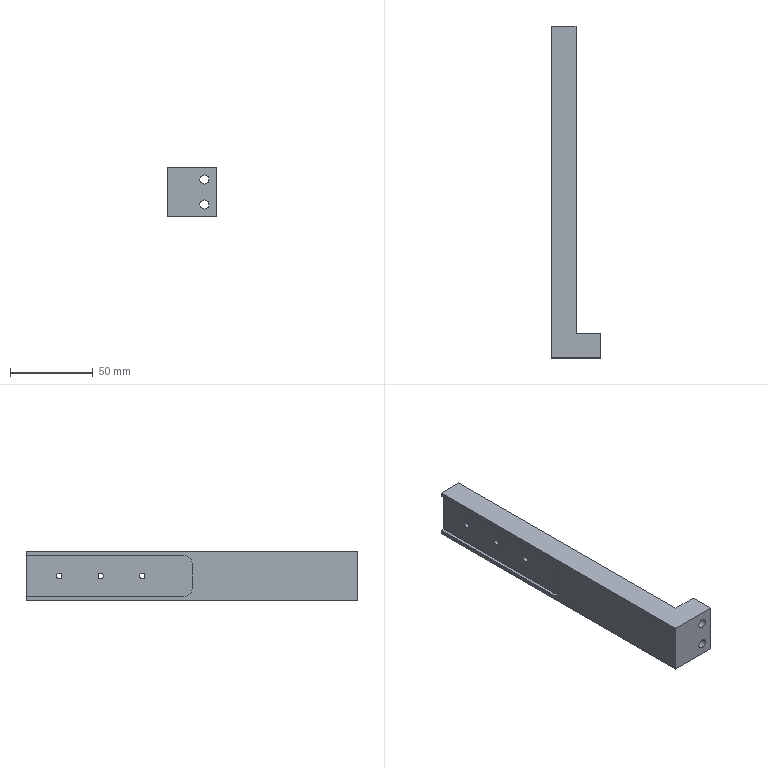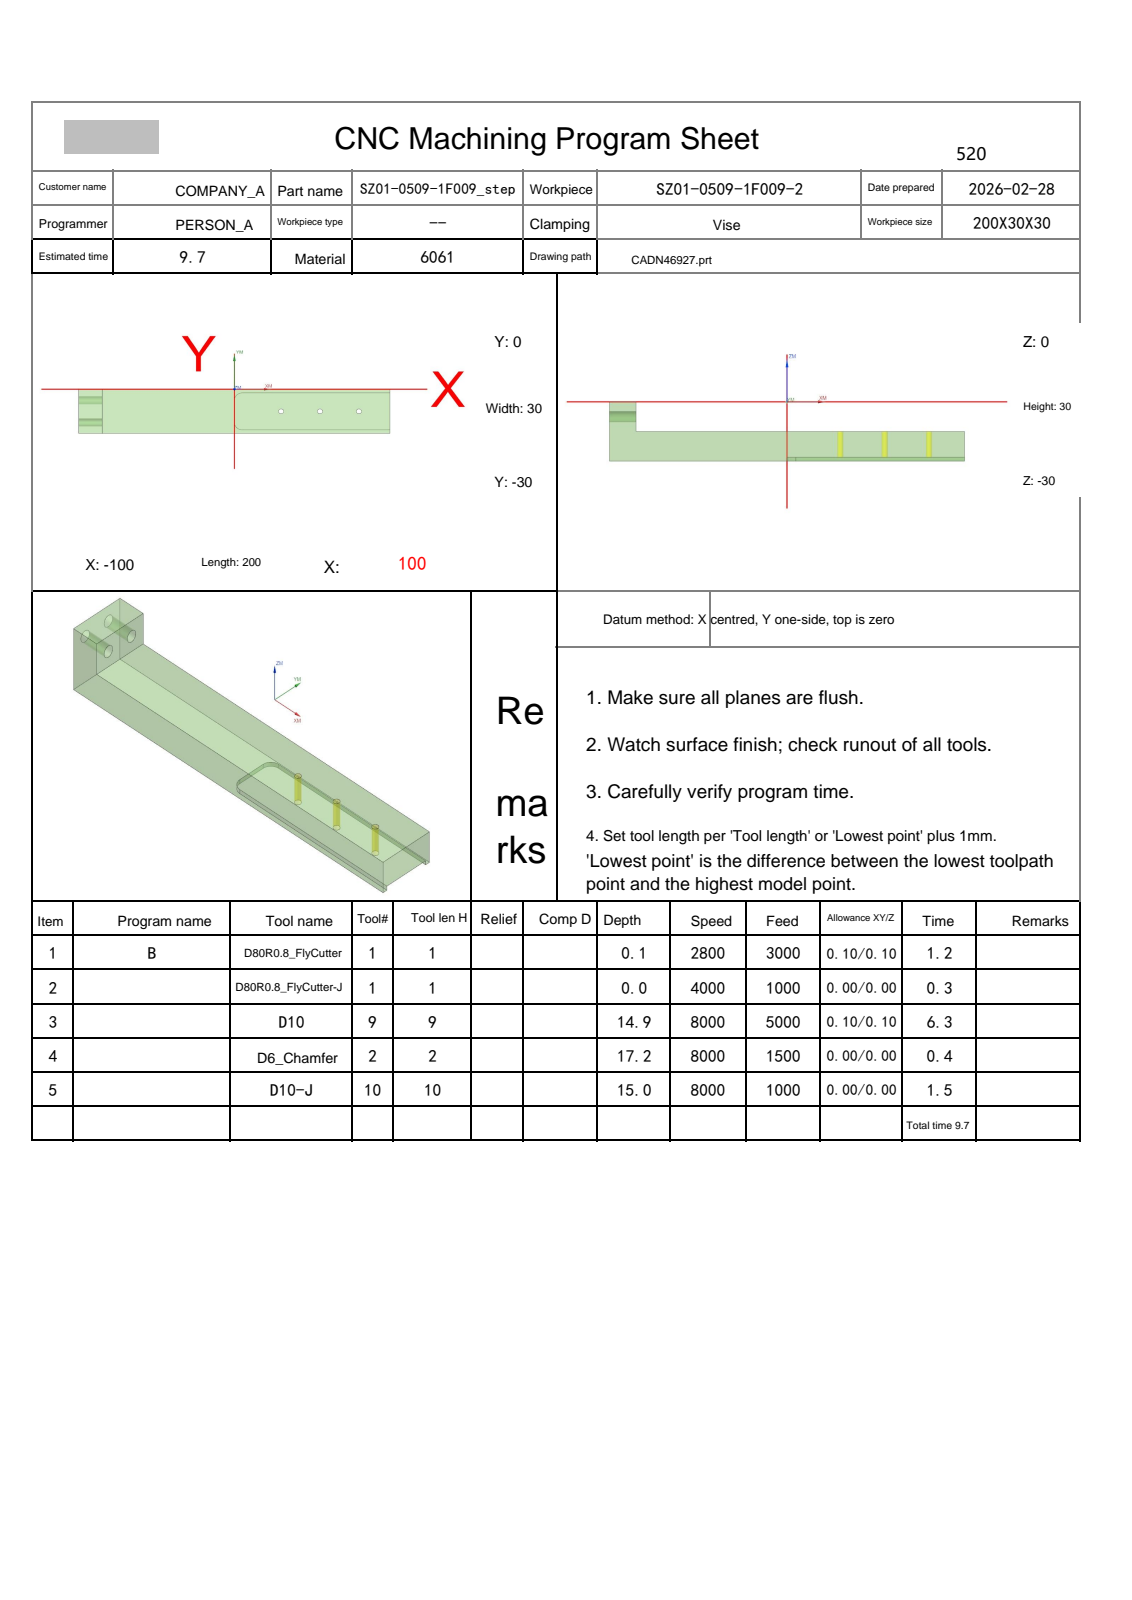NC program | NX | posted by the shop | part box 30 x 200 x 30 mm
Lines 2719 to 2890 of 2890:
N4 T02 M06
(D6_Chamfer  D=6. R=0. H=02 ce=0.00 di=0.10)
G00 G90 G54 X80. Y-15. M03 S8000
G43 H02 Z50.
M08
G98 G81 X80. Y-15. Z-17.2 R-12. F1000.
X55.
X30.
G80
G00 Z50.
G00 G90 X-83.773 Y-14.614 M03 S6500
Z50.
Z.172
G01 Z-1.2 F1500.
G03 X-83.973 Y-14.9 I1.532 J-1.286
G01 X-84.003 Y-14.946
X-84. Y-15.
Y-30.
G02 X-85. Y-31. I-1. J0.0
G01 X-100.
G02 X-101. Y-30. I0.0 J1.
G01 Y0.0
G02 X-100. Y1. I1. J0.0
G01 X-85.
G02 X-84. Y0.0 I0.0 J-1.
G01 Y-15.
X-84.003 Y-15.054
X-83.973 Y-15.1
G03 X-83.773 Y-15.386 I1.732 J1.
G01 Z.172
G00 Z10.
X-81.961 Y1.045
Z-1.815
G01 Z-16.2
X-81.904 Y1.005
X-81.884 Y1.
X100.
G02 X101. Y0.0 I0.0 J-1.
G01 Y-30.
G02 X100. Y-31. I-1. J0.0
G01 X-81.884
X-81.904 Y-31.005
X-81.961 Y-31.045
Z-1.815
G00 Z10.
X29.581 Y-15.494
Z-14.595
G01 Z-16.2
G03 X29.897 Y-15.641 I1. J1.732
G01 X29.947 Y-15.662
X30. Y-15.65
G03 X30.65 Y-15. I0.0 J.65
X30. Y-14.35 I-.65 J0.0
X29.35 Y-15. I0.0 J-.65
X30. Y-15.65 I.65 J0.0
G01 X30.053 Y-15.662
X30.103 Y-15.641
G03 X30.419 Y-15.494 I-.684 J1.879
G01 Z-14.595
G00 Z10.
X54.581
Z-14.595
G01 Z-16.2
G03 X54.897 Y-15.641 I1. J1.732
G01 X54.947 Y-15.662
X55. Y-15.65
G03 X55.65 Y-15. I0.0 J.65
X55. Y-14.35 I-.65 J0.0
X54.35 Y-15. I0.0 J-.65
X55. Y-15.65 I.65 J0.0
G01 X55.053 Y-15.662
X55.103 Y-15.641
G03 X55.419 Y-15.494 I-.684 J1.879
G01 Z-14.595
G00 Z10.
X79.581
Z-14.595
G01 Z-16.2
G03 X79.897 Y-15.641 I1. J1.732
G01 X79.947 Y-15.662
X80. Y-15.65
G03 X80.65 Y-15. I0.0 J.65
X80. Y-14.35 I-.65 J0.0
X79.35 Y-15. I0.0 J-.65
X80. Y-15.65 I.65 J0.0
G01 X80.053 Y-15.662
X80.103 Y-15.641
G03 X80.419 Y-15.494 I-.684 J1.879
G01 Z-14.595
G00 Z50.
G91 G28 Z0.0
M05
M09
G91 G28 Z0.0
M01
N5 T10 M06
(D10-J  D=10. R=0. H=10 ce=0.40 di=0.00)
G00 G90 G54 X8.7 Y7. M03 S8000
G43 H10 Z14.5
M08
Z-13.5
G01 Z-15. F1000.
Y3.
G03 X10.7 Y1. I2. J0.0
G01 X96.
X100.004
G02 X101. Y.004 I-.004 J-1.
G01 Y-30.004
G02 X100.004 Y-31. I-1. J.004
G01 X-78.604
G02 X-79.6 Y-30.004 I.004 J1.
G01 Y.004
G02 X-78.604 Y1. I1. J-.004
G01 X12.787
G02 X13.492 Y.708 I-.001 J-1.
G01 X17.908 Y-3.708
G03 X18.614 Y-4. I.707 J.708
G01 X95.004
G02 X96. Y-4.996 I-.004 J-1.
G01 Y-25.004
G02 X95.004 Y-26. I-1. J.004
G01 X-73.604
G02 X-74.6 Y-25.004 I.004 J1.
G01 Y-4.996
G02 X-73.604 Y-4. I1. J-.004
G01 X12.787
G02 X13.492 Y-4.292 I-.001 J-1.
G01 X17.908 Y-8.708
G03 X18.614 Y-9. I.707 J.708
G01 X90.004
G02 X91. Y-9.996 I-.004 J-1.
G01 Y-20.004
G02 X90.004 Y-21. I-1. J.004
G01 X-68.604
G02 X-69.6 Y-20.004 I.004 J1.
G01 Y-9.996
G02 X-68.604 Y-9. I1. J-.004
G01 X12.786
G02 X13.492 Y-9.292 I-.001 J-1.
G01 X17.908 Y-13.708
G03 X18.614 Y-14. I.707 J.708
G01 X85.005
G02 X86. Y-15. I-.005 J-1.
G01 Y-15.005
G02 X85.005 Y-16. I-1. J.005
G01 X-63.605
G02 X-64.6 Y-15. I.005 J1.
G01 Y-14.995
G02 X-63.605 Y-14. I1. J-.005
G01 X15.7
X16.7
G03 X18.7 Y-12. I0.0 J2.
G01 Z-13.5
G00 Z14.5
G00 G90 X-77.801 Y7. M03 S8000
Z14.5
Z-14.
G01 Z-15. F1000.
G41 D10
X-78.001
G03 X-80. Y5. I.001 J-2.
G01 Y-35.
G03 X-78. Y-37. I2. J0.0
G01 G40 X-77.8
Z-14.
G00 Z14.5
M05
M09
G91 G28 Z0.0
G91 G28 Y0.0
M30
%